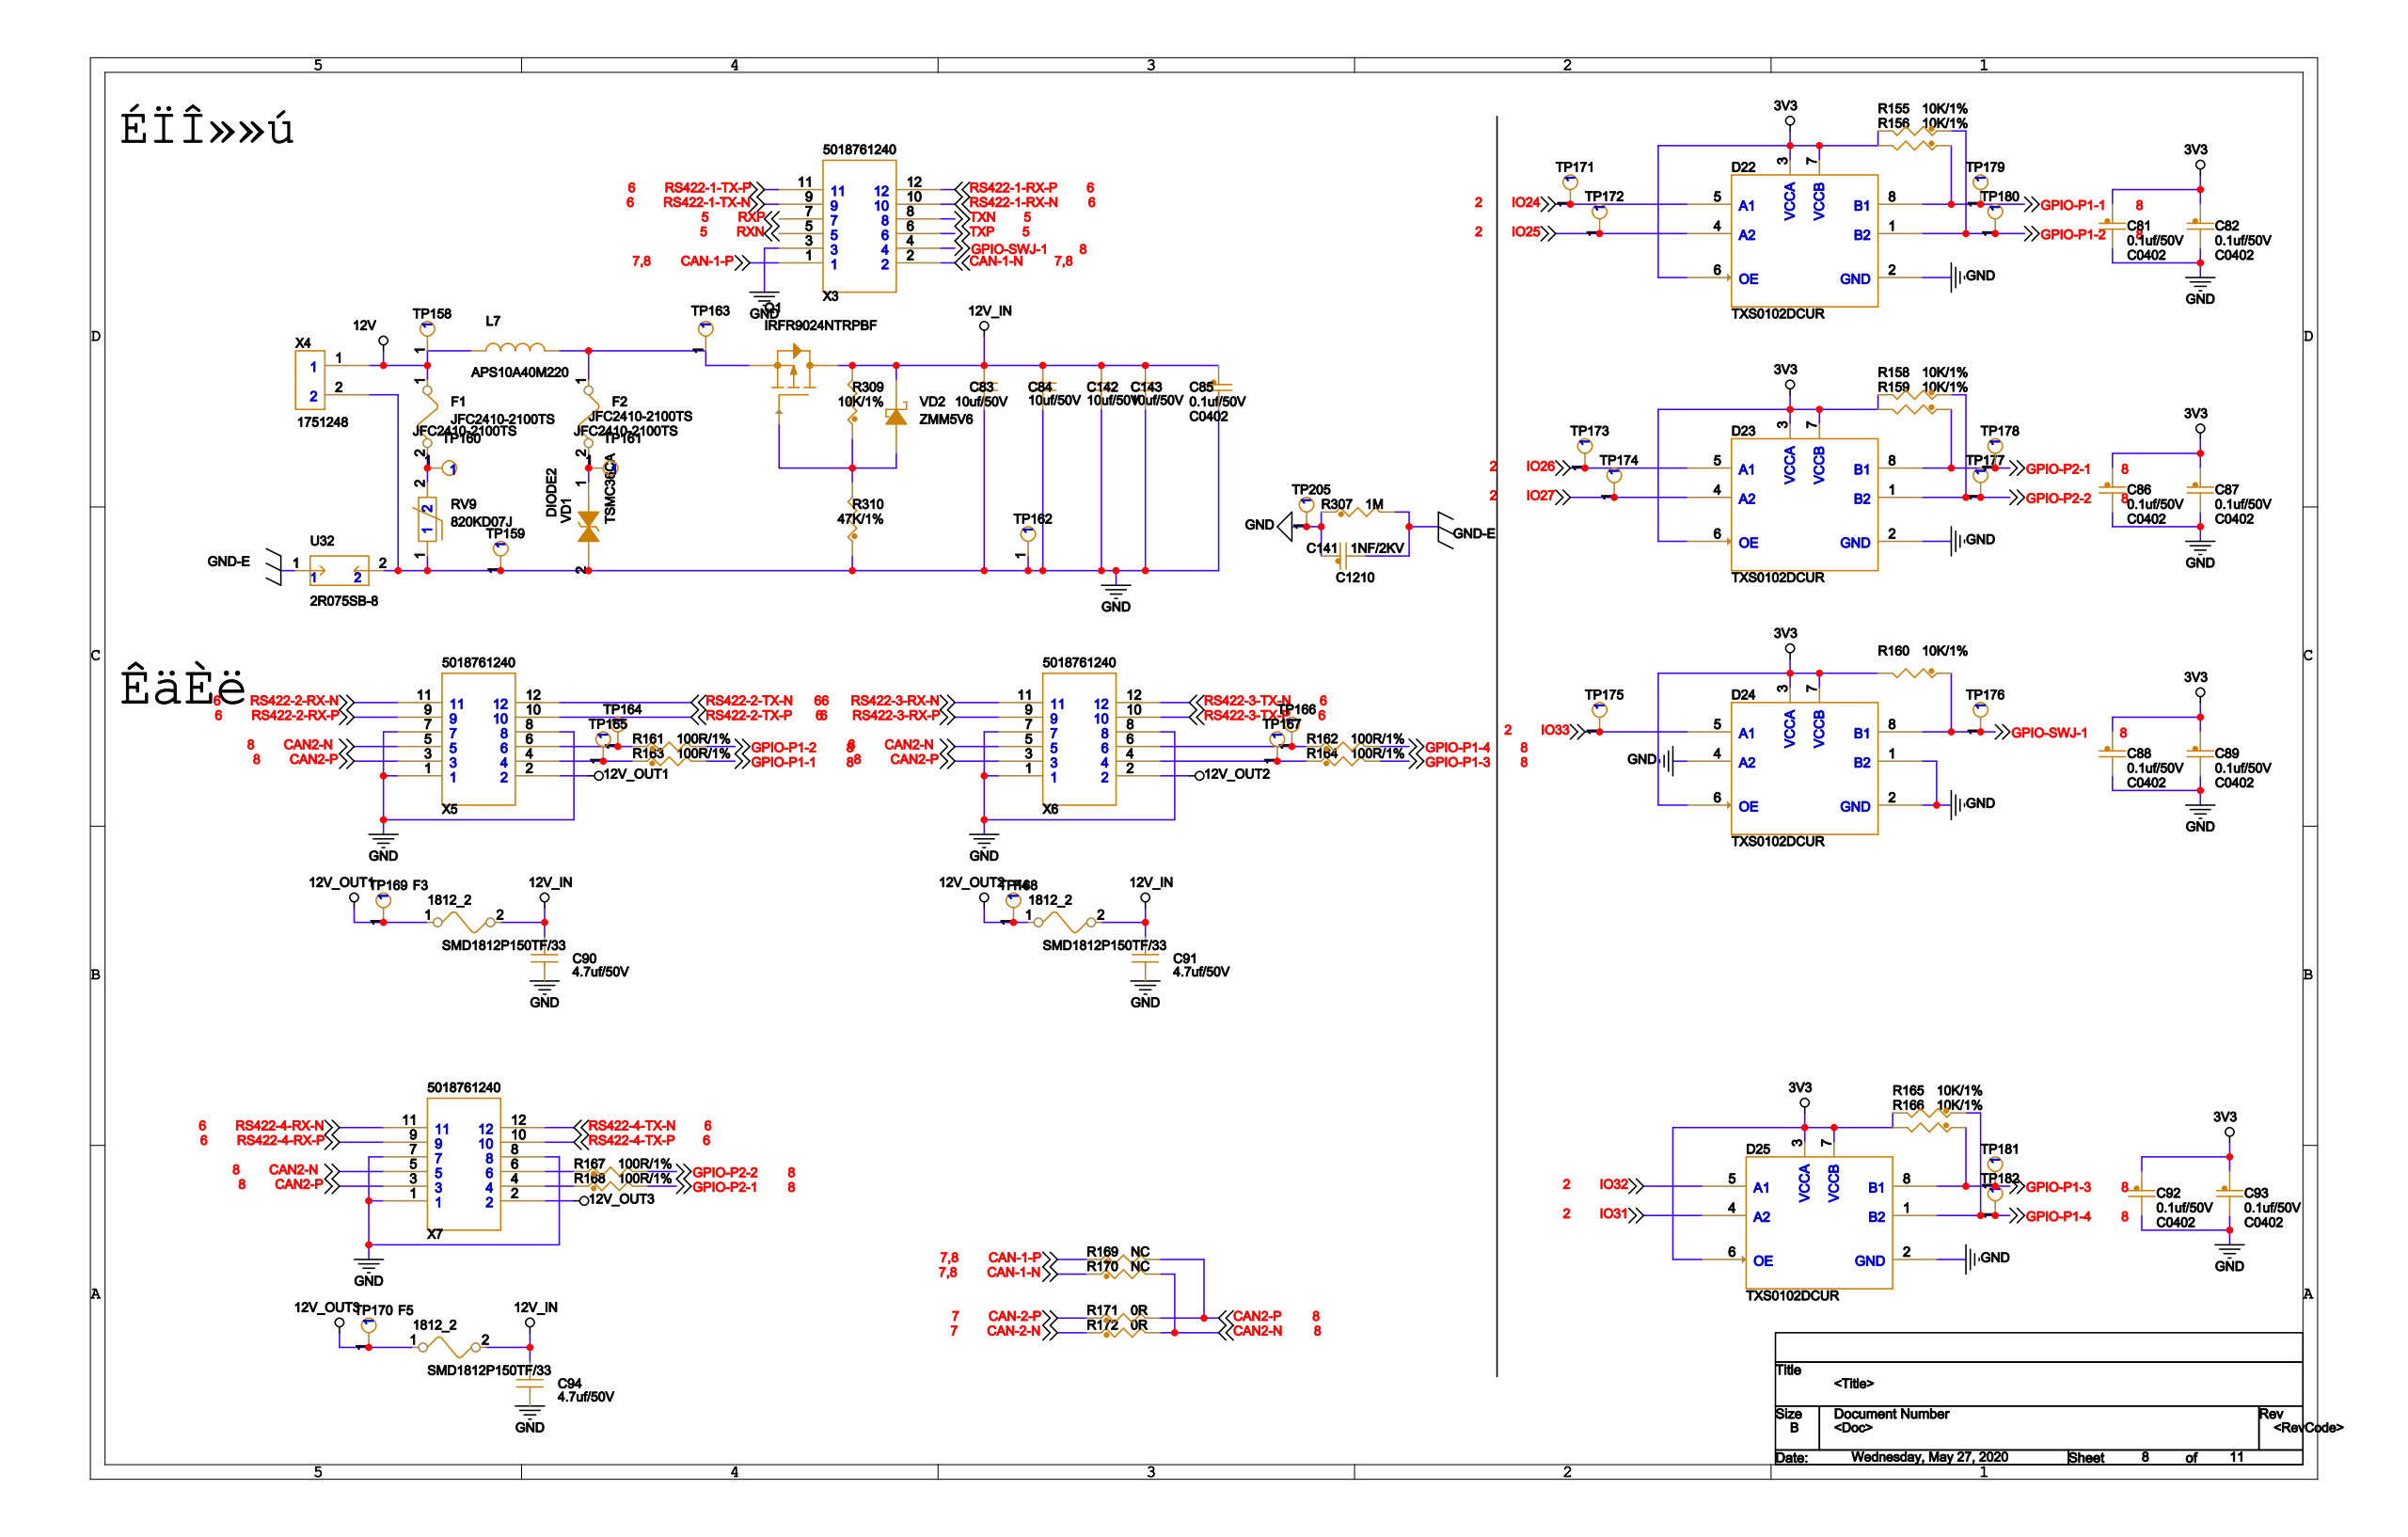Circuit board | Cadence Allegro | 521 parts | 239 nets | one sheet of the schematic
Parts on this sheet (reference | value | footprint):
C81 | 0.1uf/50V | C0402
C82 | 0.1uf/50V | C0402
C83 | 10uf/50V | C0805
C84 | 10uf/50V | C0805
C85 | 0.1uf/50V | C0402
C86 | 0.1uf/50V | C0402
C87 | 0.1uf/50V | C0402
C88 | 0.1uf/50V | C0402
C89 | 0.1uf/50V | C0402
C90 | 4.7uf/50V | C0805
C91 | 4.7uf/50V | C0805
C92 | 0.1uf/50V | C0402
C93 | 0.1uf/50V | C0402
C94 | 4.7uf/50V | C0805
C141 | 1NF/2KV | C1210
C142 | 10uf/50V | C0805
C143 | 10uf/50V | C0805
D22 | TXS0102DCUR | VSSOP8
D23 | TXS0102DCUR | VSSOP8
D24 | TXS0102DCUR | VSSOP8
D25 | TXS0102DCUR | VSSOP8
F1 | JFC2410-2100TS | JFC2410-2100TS
F2 | JFC2410-2100TS | JFC2410-2100TS
F3 | SMD1812P150TF/33 | 1812_2
F4 | SMD1812P150TF/33 | 1812_2
F5 | SMD1812P150TF/33 | 1812_2
L7 | APS10A40M220 | SM_IND_10X10
Q1 | IRFR9024NTRPBF | TO252-2
R155 | 10K/1% | 0402
R156 | 10K/1% | 0402
R158 | 10K/1% | 0402
R159 | 10K/1% | 0402
R160 | 10K/1% | 0402
R161 | 100R/1% | 0603
R162 | 100R/1% | 0603
R163 | 100R/1% | 0603
R164 | 100R/1% | 0603
R165 | 10K/1% | 0402
R166 | 10K/1% | 0402
R167 | 100R/1% | 0603
R168 | 100R/1% | 0603
R169 | NC | 0603
R170 | NC | 0603
R171 | 0R | 0603
R172 | 0R | 0603
R307 | 1M | 1206
R309 | 10K/1% | 0603
R310 | 47K/1% | 0603
RV9 | 820KD07J | 10D151K
TP158 | TESTPOINT | TESTPOINT-33MIL
TP159 | TESTPOINT | TESTPOINT-33MIL
TP160 | TESTPOINT | TESTPOINT-33MIL
TP161 | TESTPOINT | TESTPOINT-33MIL
TP162 | TESTPOINT | TESTPOINT-33MIL
TP163 | TESTPOINT | TESTPOINT-33MIL
TP164 | TESTPOINT | TESTPOINT-33MIL
TP166 | TESTPOINT | TESTPOINT-33MIL
TP168 | TESTPOINT | TESTPOINT-33MIL
TP169 | TESTPOINT | TESTPOINT-33MIL
TP170 | TESTPOINT | TESTPOINT-33MIL
TP171 | TESTPOINT | TESTPOINT-33MIL
TP172 | TESTPOINT | TESTPOINT-33MIL
TP173 | TESTPOINT | TESTPOINT-33MIL
TP174 | TESTPOINT | TESTPOINT-33MIL
TP175 | TESTPOINT | TESTPOINT-33MIL
TP176 | TESTPOINT | TESTPOINT-33MIL
TP177 | TESTPOINT | TESTPOINT-33MIL
TP178 | TESTPOINT | TESTPOINT-33MIL
TP179 | TESTPOINT | TESTPOINT-33MIL
TP180 | TESTPOINT | TESTPOINT-33MIL
TP181 | TESTPOINT | TESTPOINT-33MIL
TP182 | TESTPOINT | TESTPOINT-33MIL
TP205 | TESTPOINT | TESTPOINT-33MIL
U32 | 2R075SB-8 | 2R075SB
VD2 | ZMM5V6 | DIODE2
X3 | 5018761240 | 5018761240
X4 | 1751248 | EDG-35-2P
X5 | 5018761240 | 5018761240
X6 | 5018761240 | 5018761240
X7 | 5018761240 | 5018761240
Nets of these parts (net: part-pin ...):
GND: C81-2 C82-2 C83-2 C84-2 C85-2 C86-2 C87-2 C88-2 C89-2 C90-2 C91-2 C92-2 C93-2 C94-2 C141-1 C142-2 C143-2 D22-2 D23-2 D24-1 D24-2 D24-4 D25-2 R307-1 R310-1 RV9-1 TP159-1 TP162-1 TP205-1 U32-2 X3-3 X4-2 X5-1 X5-7 X5-8 X6-1 X6-7 X6-8 X7-1 X7-7 X7-8
12V: F1-1 L7-1 TP158-1 X4-1
N7596674: F2-1 L7-2 Q1-2 TP163-1
12V_IN: C83-1 C84-1 C85-1 C90-1 C91-1 C94-1 C142-1 C143-1 F3-2 F4-2 F5-2 Q1-3 R309-2 VD2-2
N7883668: Q1-1 R309-1 R310-2 VD2-1
N7655168: F1-2 RV9-2 TP160-1
3V3: C81-1 C82-1 C86-1 C87-1 C88-1 C89-1 C92-1 C93-1 D22-3 D22-6 D22-7 D23-3 D23-6 D23-7 D24-3 D24-6 D24-7 D25-3 D25-6 D25-7 R155-2 R156-2 R158-2 R159-2 R160-2 R165-2 R166-2
GND-E: C141-2 R307-2 U32-1
RS422-2-TX-N: X5-12
RS422-3-RX-P: X6-9
RS422-3-RX-N: X6-11
RS422-3-TX-P: X6-10
RS422-3-TX-N: X6-12
RS422-4-RX-P: X7-9
RS422-4-RX-N: X7-11
RS422-4-TX-N: X7-12
RS422-4-TX-P: X7-10
CAN-1-N: R170-1 X3-2
CAN-1-P: R169-1 X3-1
CAN-2-N: R172-1
CAN-2-P: R171-1
N7655230: F2-2 TP161-1
N7378094: R161-1 TP164-1 X5-6
N7378096: R163-1 X5-4
N7379563: R162-1 TP166-1 X6-6
N7379567: R164-1 X6-4
12V_OUT2: F4-1 TP168-1 X6-2
12V_OUT1: F3-1 TP169-1 X5-2
12V_OUT3: F5-1 TP170-1 X7-2
IO24: D22-5 TP171-1
IO25: D22-4 TP172-1
IO26: D23-5 TP173-1
IO27: D23-4 TP174-1
IO33: D24-5 TP175-1
GPIO-SWJ-1: D24-8 R160-1 TP176-1 X3-4
GPIO-P2-2: D23-1 R158-1 R167-2 TP177-1
GPIO-P2-1: D23-8 R159-1 R168-2 TP178-1
GPIO-P1-1: D22-8 R156-1 R163-2 TP179-1
GPIO-P1-2: D22-1 R155-1 R161-2 TP180-1
GPIO-P1-3: D25-8 R164-2 R166-1 TP181-1
GPIO-P1-4: D25-1 R162-2 R165-1 TP182-1
RS422-2-RX-P: X5-9
RS422-2-RX-N: X5-11
RS422-2-TX-P: X5-10
RXN: X3-5
RXP: X3-7
RS422-1-RX-P: X3-12
RS422-1-RX-N: X3-10
RS422-1-TX-P: X3-11
RS422-1-TX-N: X3-9
TXN: X3-8
TXP: X3-6
IO32: D25-5
IO31: D25-4
CAN2-P: R169-2 R171-2 X5-3 X6-3 X7-3
CAN2-N: R170-2 R172-2 X5-5 X6-5 X7-5
N7380640: R167-1 X7-6
N7380644: R168-1 X7-4